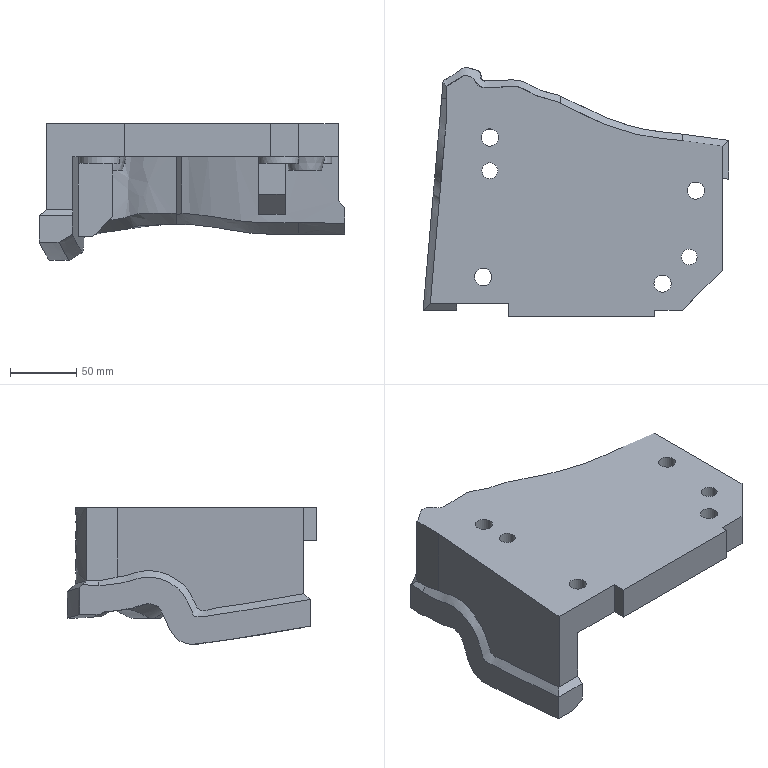Part | NX | features solid 2 | 1 solid | 81 faces | box 230.338 x 188.137 x 103.022 mm | volume 1356148 mm3 | plane 42 | spline 23 | cylinder 14 | cone 2 | commonest cylinder face diameters 13 x6 30 x6 12 x2